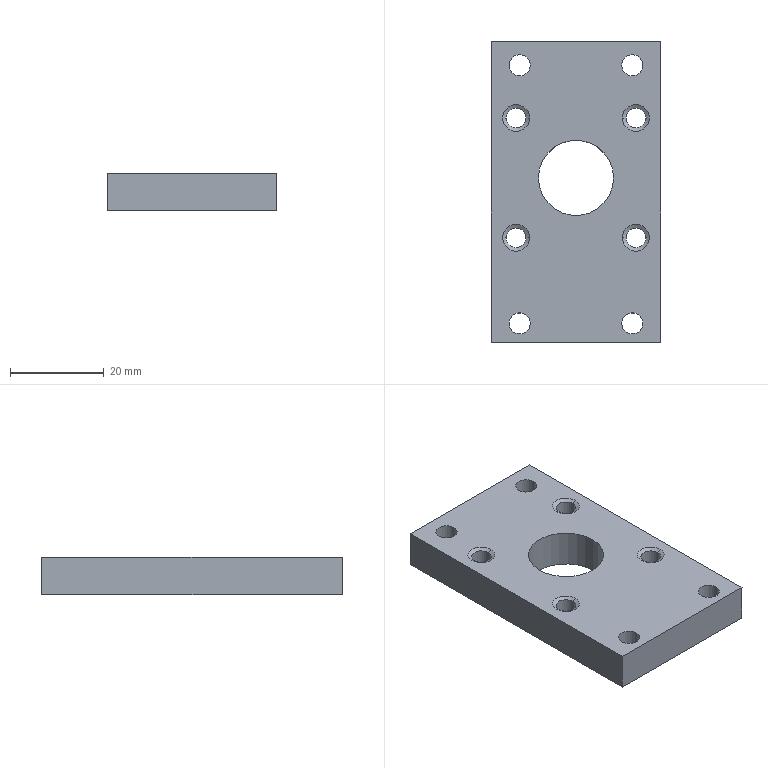Part | NX | 1 solid | 32 faces | box 36.002 x 64 x 8.011 mm | volume 15861 mm3 | cylinder 18 | cone 8 | plane 6 | commonest cylinder face diameters 4.2 x8 4.5 x8 16 x2
STEP:
#1=CARTESIAN_POINT('',(1234.583,117.5,67.602));
#2=VERTEX_POINT('',#1);
#3=CARTESIAN_POINT('',(1198.583,117.5,67.613));
#4=VERTEX_POINT('',#3);
#5=CARTESIAN_POINT('',(1211.755,117.5,67.609));
#6=DIRECTION('',(-1.,0.,0.0003046));
#7=VECTOR('',#6,1000.);
#8=LINE('',#5,#7);
#9=EDGE_CURVE('',#2,#4,#8,.T.);
#10=ORIENTED_EDGE('',*,*,#9,.F.);
#11=CARTESIAN_POINT('',(1234.585,117.5,75.602));
#12=VERTEX_POINT('',#11);
#13=CARTESIAN_POINT('',(1234.582,117.5,65.602));
#14=DIRECTION('',(0.0003046,0.,1.));
#15=VECTOR('',#14,1000.);
#16=LINE('',#13,#15);
#17=EDGE_CURVE('',#2,#12,#16,.T.);
#18=ORIENTED_EDGE('',*,*,#17,.T.);
#19=CARTESIAN_POINT('',(1198.585,117.5,75.613));
#20=VERTEX_POINT('',#19);
#21=CARTESIAN_POINT('',(1211.758,117.5,75.609));
#22=DIRECTION('',(-1.,0.,0.0003046));
#23=VECTOR('',#22,1000.);
#24=LINE('',#21,#23);
#25=EDGE_CURVE('',#12,#20,#24,.T.);
#26=ORIENTED_EDGE('',*,*,#25,.T.);
#27=CARTESIAN_POINT('',(1198.582,117.5,65.613));
#28=DIRECTION('',(-0.0003046,0.,-1.));
#29=VECTOR('',#28,1000.);
#30=LINE('',#27,#29);
#31=EDGE_CURVE('',#20,#4,#30,.T.);
#32=ORIENTED_EDGE('',*,*,#31,.T.);
#33=EDGE_LOOP('',(#10,#18,#26,#32));
#34=FACE_BOUND('',#33,.T.);
#35=CARTESIAN_POINT('',(1236.582,117.5,65.601));
#36=DIRECTION('',(0.,-1.,0.));
#37=DIRECTION('',(0.,0.,-1.));
#38=AXIS2_PLACEMENT_3D('',#35,#36,#37);
#39=PLANE('',#38);
#40=ADVANCED_FACE('',(#34),#39,.T.);
#41=CARTESIAN_POINT('',(1234.583,181.5,67.602));
#42=VERTEX_POINT('',#41);
#43=CARTESIAN_POINT('',(1234.583,131.898,67.602));
#44=DIRECTION('',(0.,-1.,0.));
#45=VECTOR('',#44,1000.);
#46=LINE('',#43,#45);
#47=EDGE_CURVE('',#42,#2,#46,.T.);
#48=ORIENTED_EDGE('',*,*,#47,.F.);
#49=CARTESIAN_POINT('',(1234.585,181.5,75.602));
#50=VERTEX_POINT('',#49);
#51=CARTESIAN_POINT('',(1234.582,181.5,65.602));
#52=DIRECTION('',(0.0003046,0.,1.));
#53=VECTOR('',#52,1000.);
#54=LINE('',#51,#53);
#55=EDGE_CURVE('',#42,#50,#54,.T.);
#56=ORIENTED_EDGE('',*,*,#55,.T.);
#57=CARTESIAN_POINT('',(1234.585,131.898,75.602));
#58=DIRECTION('',(0.,-1.,0.));
#59=VECTOR('',#58,1000.);
#60=LINE('',#57,#59);
#61=EDGE_CURVE('',#50,#12,#60,.T.);
#62=ORIENTED_EDGE('',*,*,#61,.T.);
#63=ORIENTED_EDGE('',*,*,#17,.F.);
#64=EDGE_LOOP('',(#48,#56,#62,#63));
#65=FACE_BOUND('',#64,.T.);
#66=CARTESIAN_POINT('',(1234.582,127.5,65.602));
#67=DIRECTION('',(1.,0.,-0.0003046));
#68=DIRECTION('',(0.,-1.,0.));
#69=AXIS2_PLACEMENT_3D('',#66,#67,#68);
#70=PLANE('',#69);
#71=ADVANCED_FACE('',(#65),#70,.T.);
#72=CARTESIAN_POINT('',(1198.583,181.5,67.613));
#73=VERTEX_POINT('',#72);
#74=CARTESIAN_POINT('',(1211.755,181.5,67.609));
#75=DIRECTION('',(1.,0.,-0.0003046));
#76=VECTOR('',#75,1000.);
#77=LINE('',#74,#76);
#78=EDGE_CURVE('',#73,#42,#77,.T.);
#79=ORIENTED_EDGE('',*,*,#78,.F.);
#80=CARTESIAN_POINT('',(1198.585,181.5,75.613));
#81=VERTEX_POINT('',#80);
#82=CARTESIAN_POINT('',(1198.582,181.5,65.613));
#83=DIRECTION('',(-0.0003046,0.,-1.));
#84=VECTOR('',#83,1000.);
#85=LINE('',#82,#84);
#86=EDGE_CURVE('',#81,#73,#85,.T.);
#87=ORIENTED_EDGE('',*,*,#86,.F.);
#88=CARTESIAN_POINT('',(1211.758,181.5,75.609));
#89=DIRECTION('',(1.,0.,-0.0003046));
#90=VECTOR('',#89,1000.);
#91=LINE('',#88,#90);
#92=EDGE_CURVE('',#81,#50,#91,.T.);
#93=ORIENTED_EDGE('',*,*,#92,.T.);
#94=ORIENTED_EDGE('',*,*,#55,.F.);
#95=EDGE_LOOP('',(#79,#87,#93,#94));
#96=FACE_BOUND('',#95,.T.);
#97=CARTESIAN_POINT('',(1196.582,181.5,65.614));
#98=DIRECTION('',(0.,1.,0.));
#99=DIRECTION('',(0.,0.,-1.));
#100=AXIS2_PLACEMENT_3D('',#97,#98,#99);
#101=PLANE('',#100);
#102=ADVANCED_FACE('',(#96),#101,.T.);
#103=CARTESIAN_POINT('',(1198.583,131.898,67.613));
#104=DIRECTION('',(0.,1.,0.));
#105=VECTOR('',#104,1000.);
#106=LINE('',#103,#105);
#107=EDGE_CURVE('',#4,#73,#106,.T.);
#108=ORIENTED_EDGE('',*,*,#107,.F.);
#109=ORIENTED_EDGE('',*,*,#31,.F.);
#110=CARTESIAN_POINT('',(1198.585,131.898,75.613));
#111=DIRECTION('',(0.,1.,0.));
#112=VECTOR('',#111,1000.);
#113=LINE('',#110,#112);
#114=EDGE_CURVE('',#20,#81,#113,.T.);
#115=ORIENTED_EDGE('',*,*,#114,.T.);
#116=ORIENTED_EDGE('',*,*,#86,.T.);
#117=EDGE_LOOP('',(#108,#109,#115,#116));
#118=FACE_BOUND('',#117,.T.);
#119=CARTESIAN_POINT('',(1198.582,117.5,65.613));
#120=DIRECTION('',(-1.,0.,0.0003046));
#121=DIRECTION('',(0.,1.,0.));
#122=AXIS2_PLACEMENT_3D('',#119,#120,#121);
#123=PLANE('',#122);
#124=ADVANCED_FACE('',(#118),#123,.T.);
#125=ORIENTED_EDGE('',*,*,#61,.F.);
#126=ORIENTED_EDGE('',*,*,#92,.F.);
#127=ORIENTED_EDGE('',*,*,#114,.F.);
#128=ORIENTED_EDGE('',*,*,#25,.F.);
#129=EDGE_LOOP('',(#125,#126,#127,#128));
#130=FACE_BOUND('',#129,.T.);
#131=CARTESIAN_POINT('',(1224.585,152.5,75.605));
#132=VERTEX_POINT('',#131);
#133=CARTESIAN_POINT('',(1208.585,152.5,75.61));
#134=VERTEX_POINT('',#133);
#135=CARTESIAN_POINT('',(1216.585,152.5,75.608));
#136=DIRECTION('',(-0.0003046,0.,-1.));
#137=DIRECTION('',(-1.,0.,0.0003046));
#138=AXIS2_PLACEMENT_3D('',#135,#136,#137);
#139=CIRCLE('',#138,8.);
#140=EDGE_CURVE('',#132,#134,#139,.T.);
#141=ORIENTED_EDGE('',*,*,#140,.T.);
#142=CARTESIAN_POINT('',(1216.585,152.5,75.608));
#143=DIRECTION('',(-0.0003046,0.,-1.));
#144=DIRECTION('',(-1.,0.,0.0003046));
#145=AXIS2_PLACEMENT_3D('',#142,#143,#144);
#146=CIRCLE('',#145,8.);
#147=EDGE_CURVE('',#134,#132,#146,.T.);
#148=ORIENTED_EDGE('',*,*,#147,.T.);
#149=EDGE_LOOP('',(#141,#148));
#150=FACE_BOUND('',#149,.T.);
#151=CARTESIAN_POINT('',(1226.475,165.25,75.605));
#152=VERTEX_POINT('',#151);
#153=CARTESIAN_POINT('',(1232.195,165.25,75.603));
#154=VERTEX_POINT('',#153);
#155=CARTESIAN_POINT('',(1229.335,165.25,75.604));
#156=DIRECTION('',(0.0003046,0.,1.));
#157=DIRECTION('',(1.,0.,-0.0003046));
#158=AXIS2_PLACEMENT_3D('',#155,#156,#157);
#159=CIRCLE('',#158,2.86);
#160=EDGE_CURVE('',#152,#154,#159,.T.);
#161=ORIENTED_EDGE('',*,*,#160,.F.);
#162=CARTESIAN_POINT('',(1229.335,165.25,75.604));
#163=DIRECTION('',(0.0003046,0.,1.));
#164=DIRECTION('',(1.,0.,-0.0003046));
#165=AXIS2_PLACEMENT_3D('',#162,#163,#164);
#166=CIRCLE('',#165,2.86);
#167=EDGE_CURVE('',#154,#152,#166,.T.);
#168=ORIENTED_EDGE('',*,*,#167,.F.);
#169=EDGE_LOOP('',(#161,#168));
#170=FACE_BOUND('',#169,.T.);
#171=CARTESIAN_POINT('',(1232.195,139.75,75.603));
#172=VERTEX_POINT('',#171);
#173=CARTESIAN_POINT('',(1226.475,139.75,75.605));
#174=VERTEX_POINT('',#173);
#175=CARTESIAN_POINT('',(1229.335,139.75,75.604));
#176=DIRECTION('',(0.0003046,0.,1.));
#177=DIRECTION('',(1.,0.,-0.0003046));
#178=AXIS2_PLACEMENT_3D('',#175,#176,#177);
#179=CIRCLE('',#178,2.86);
#180=EDGE_CURVE('',#172,#174,#179,.T.);
#181=ORIENTED_EDGE('',*,*,#180,.F.);
#182=CARTESIAN_POINT('',(1229.335,139.75,75.604));
#183=DIRECTION('',(0.0003046,0.,1.));
#184=DIRECTION('',(1.,0.,-0.0003046));
#185=AXIS2_PLACEMENT_3D('',#182,#183,#184);
#186=CIRCLE('',#185,2.86);
#187=EDGE_CURVE('',#174,#172,#186,.T.);
#188=ORIENTED_EDGE('',*,*,#187,.F.);
#189=EDGE_LOOP('',(#181,#188));
#190=FACE_BOUND('',#189,.T.);
#191=CARTESIAN_POINT('',(1226.335,121.5,75.605));
#192=VERTEX_POINT('',#191);
#193=CARTESIAN_POINT('',(1230.835,121.5,75.603));
#194=VERTEX_POINT('',#193);
#195=CARTESIAN_POINT('',(1228.585,121.5,75.604));
#196=DIRECTION('',(0.0003046,0.,1.));
#197=DIRECTION('',(1.,0.,-0.0003046));
#198=AXIS2_PLACEMENT_3D('',#195,#196,#197);
#199=CIRCLE('',#198,2.25);
#200=EDGE_CURVE('',#192,#194,#199,.T.);
#201=ORIENTED_EDGE('',*,*,#200,.F.);
#202=CARTESIAN_POINT('',(1228.585,121.5,75.604));
#203=DIRECTION('',(0.0003046,0.,1.));
#204=DIRECTION('',(1.,0.,-0.0003046));
#205=AXIS2_PLACEMENT_3D('',#202,#203,#204);
#206=CIRCLE('',#205,2.25);
#207=EDGE_CURVE('',#194,#192,#206,.T.);
#208=ORIENTED_EDGE('',*,*,#207,.F.);
#209=EDGE_LOOP('',(#201,#208));
#210=FACE_BOUND('',#209,.T.);
#211=CARTESIAN_POINT('',(1202.335,121.5,75.612));
#212=VERTEX_POINT('',#211);
#213=CARTESIAN_POINT('',(1206.835,121.5,75.611));
#214=VERTEX_POINT('',#213);
#215=CARTESIAN_POINT('',(1204.585,121.5,75.611));
#216=DIRECTION('',(0.0003046,0.,1.));
#217=DIRECTION('',(1.,0.,-0.0003046));
#218=AXIS2_PLACEMENT_3D('',#215,#216,#217);
#219=CIRCLE('',#218,2.25);
#220=EDGE_CURVE('',#212,#214,#219,.T.);
#221=ORIENTED_EDGE('',*,*,#220,.F.);
#222=CARTESIAN_POINT('',(1204.585,121.5,75.611));
#223=DIRECTION('',(0.0003046,0.,1.));
#224=DIRECTION('',(1.,0.,-0.0003046));
#225=AXIS2_PLACEMENT_3D('',#222,#223,#224);
#226=CIRCLE('',#225,2.25);
#227=EDGE_CURVE('',#214,#212,#226,.T.);
#228=ORIENTED_EDGE('',*,*,#227,.F.);
#229=EDGE_LOOP('',(#221,#228));
#230=FACE_BOUND('',#229,.T.);
#231=CARTESIAN_POINT('',(1202.335,176.5,75.612));
#232=VERTEX_POINT('',#231);
#233=CARTESIAN_POINT('',(1206.835,176.5,75.611));
#234=VERTEX_POINT('',#233);
#235=CARTESIAN_POINT('',(1204.585,176.5,75.611));
#236=DIRECTION('',(0.0003046,0.,1.));
#237=DIRECTION('',(1.,0.,-0.0003046));
#238=AXIS2_PLACEMENT_3D('',#235,#236,#237);
#239=CIRCLE('',#238,2.25);
#240=EDGE_CURVE('',#232,#234,#239,.T.);
#241=ORIENTED_EDGE('',*,*,#240,.F.);
#242=CARTESIAN_POINT('',(1204.585,176.5,75.611));
#243=DIRECTION('',(0.0003046,0.,1.));
#244=DIRECTION('',(1.,0.,-0.0003046));
#245=AXIS2_PLACEMENT_3D('',#242,#243,#244);
#246=CIRCLE('',#245,2.25);
#247=EDGE_CURVE('',#234,#232,#246,.T.);
#248=ORIENTED_EDGE('',*,*,#247,.F.);
#249=EDGE_LOOP('',(#241,#248));
#250=FACE_BOUND('',#249,.T.);
#251=CARTESIAN_POINT('',(1230.835,176.5,75.603));
#252=VERTEX_POINT('',#251);
#253=CARTESIAN_POINT('',(1226.335,176.5,75.605));
#254=VERTEX_POINT('',#253);
#255=CARTESIAN_POINT('',(1228.585,176.5,75.604));
#256=DIRECTION('',(0.0003046,0.,1.));
#257=DIRECTION('',(1.,0.,-0.0003046));
#258=AXIS2_PLACEMENT_3D('',#255,#256,#257);
#259=CIRCLE('',#258,2.25);
#260=EDGE_CURVE('',#252,#254,#259,.T.);
#261=ORIENTED_EDGE('',*,*,#260,.F.);
#262=CARTESIAN_POINT('',(1228.585,176.5,75.604));
#263=DIRECTION('',(0.0003046,0.,1.));
#264=DIRECTION('',(1.,0.,-0.0003046));
#265=AXIS2_PLACEMENT_3D('',#262,#263,#264);
#266=CIRCLE('',#265,2.25);
#267=EDGE_CURVE('',#254,#252,#266,.T.);
#268=ORIENTED_EDGE('',*,*,#267,.F.);
#269=EDGE_LOOP('',(#261,#268));
#270=FACE_BOUND('',#269,.T.);
#271=CARTESIAN_POINT('',(1206.695,139.75,75.611));
#272=VERTEX_POINT('',#271);
#273=CARTESIAN_POINT('',(1200.975,139.75,75.612));
#274=VERTEX_POINT('',#273);
#275=CARTESIAN_POINT('',(1203.835,139.75,75.611));
#276=DIRECTION('',(0.0003046,0.,1.));
#277=DIRECTION('',(1.,0.,-0.0003046));
#278=AXIS2_PLACEMENT_3D('',#275,#276,#277);
#279=CIRCLE('',#278,2.86);
#280=EDGE_CURVE('',#272,#274,#279,.T.);
#281=ORIENTED_EDGE('',*,*,#280,.F.);
#282=CARTESIAN_POINT('',(1203.835,139.75,75.611));
#283=DIRECTION('',(0.0003046,0.,1.));
#284=DIRECTION('',(1.,0.,-0.0003046));
#285=AXIS2_PLACEMENT_3D('',#282,#283,#284);
#286=CIRCLE('',#285,2.86);
#287=EDGE_CURVE('',#274,#272,#286,.T.);
#288=ORIENTED_EDGE('',*,*,#287,.F.);
#289=EDGE_LOOP('',(#281,#288));
#290=FACE_BOUND('',#289,.T.);
#291=CARTESIAN_POINT('',(1200.975,165.25,75.612));
#292=VERTEX_POINT('',#291);
#293=CARTESIAN_POINT('',(1206.695,165.25,75.611));
#294=VERTEX_POINT('',#293);
#295=CARTESIAN_POINT('',(1203.835,165.25,75.611));
#296=DIRECTION('',(0.0003046,0.,1.));
#297=DIRECTION('',(1.,0.,-0.0003046));
#298=AXIS2_PLACEMENT_3D('',#295,#296,#297);
#299=CIRCLE('',#298,2.86);
#300=EDGE_CURVE('',#292,#294,#299,.T.);
#301=ORIENTED_EDGE('',*,*,#300,.F.);
#302=CARTESIAN_POINT('',(1203.835,165.25,75.611));
#303=DIRECTION('',(0.0003046,0.,1.));
#304=DIRECTION('',(1.,0.,-0.0003046));
#305=AXIS2_PLACEMENT_3D('',#302,#303,#304);
#306=CIRCLE('',#305,2.86);
#307=EDGE_CURVE('',#294,#292,#306,.T.);
#308=ORIENTED_EDGE('',*,*,#307,.F.);
#309=EDGE_LOOP('',(#301,#308));
#310=FACE_BOUND('',#309,.T.);
#311=CARTESIAN_POINT('',(1211.758,131.898,75.609));
#312=DIRECTION('',(0.0003046,0.,1.));
#313=DIRECTION('',(-0.000000134,-1.,0.));
#314=AXIS2_PLACEMENT_3D('',#311,#312,#313);
#315=PLANE('',#314);
#316=ADVANCED_FACE('',(#130,#150,#170,#190,#210,#230,#250,#270,#290,#310),#315,.T.);
#317=ORIENTED_EDGE('',*,*,#140,.F.);
#318=CARTESIAN_POINT('',(1224.583,152.5,67.605));
#319=VERTEX_POINT('',#318);
#320=CARTESIAN_POINT('',(1224.585,152.5,76.62));
#321=DIRECTION('',(-0.0003046,0.,-1.));
#322=VECTOR('',#321,1000.);
#323=LINE('',#320,#322);
#324=EDGE_CURVE('',#319,#132,#323,.F.);
#325=ORIENTED_EDGE('',*,*,#324,.F.);
#326=CARTESIAN_POINT('',(1208.583,152.5,67.61));
#327=VERTEX_POINT('',#326);
#328=CARTESIAN_POINT('',(1216.583,152.5,67.608));
#329=DIRECTION('',(-0.0003046,0.,-1.));
#330=DIRECTION('',(-1.,0.,0.0003046));
#331=AXIS2_PLACEMENT_3D('',#328,#329,#330);
#332=CIRCLE('',#331,8.);
#333=EDGE_CURVE('',#319,#327,#332,.T.);
#334=ORIENTED_EDGE('',*,*,#333,.T.);
#335=CARTESIAN_POINT('',(1208.585,152.5,76.625));
#336=DIRECTION('',(-0.0003046,0.,-1.));
#337=VECTOR('',#336,1000.);
#338=LINE('',#335,#337);
#339=EDGE_CURVE('',#327,#134,#338,.F.);
#340=ORIENTED_EDGE('',*,*,#339,.T.);
#341=EDGE_LOOP('',(#317,#325,#334,#340));
#342=FACE_BOUND('',#341,.T.);
#343=CARTESIAN_POINT('',(1216.585,152.5,76.622));
#344=DIRECTION('',(-0.0003046,0.,-1.));
#345=DIRECTION('',(-1.,0.,0.0003046));
#346=AXIS2_PLACEMENT_3D('',#343,#344,#345);
#347=CYLINDRICAL_SURFACE('',#346,8.);
#348=ADVANCED_FACE('',(#342),#347,.F.);
#349=ORIENTED_EDGE('',*,*,#240,.T.);
#350=CARTESIAN_POINT('',(1206.833,176.5,67.611));
#351=VERTEX_POINT('',#350);
#352=CARTESIAN_POINT('',(1206.832,176.5,66.797));
#353=DIRECTION('',(0.0003046,0.,1.));
#354=VECTOR('',#353,1000.);
#355=LINE('',#352,#354);
#356=EDGE_CURVE('',#351,#234,#355,.T.);
#357=ORIENTED_EDGE('',*,*,#356,.F.);
#358=CARTESIAN_POINT('',(1202.333,176.5,67.612));
#359=VERTEX_POINT('',#358);
#360=CARTESIAN_POINT('',(1204.583,176.5,67.611));
#361=DIRECTION('',(0.0003046,0.,1.));
#362=DIRECTION('',(1.,0.,-0.0003046));
#363=AXIS2_PLACEMENT_3D('',#360,#361,#362);
#364=CIRCLE('',#363,2.25);
#365=EDGE_CURVE('',#359,#351,#364,.T.);
#366=ORIENTED_EDGE('',*,*,#365,.F.);
#367=CARTESIAN_POINT('',(1202.332,176.5,66.799));
#368=DIRECTION('',(0.0003046,0.,1.));
#369=VECTOR('',#368,1000.);
#370=LINE('',#367,#369);
#371=EDGE_CURVE('',#359,#232,#370,.T.);
#372=ORIENTED_EDGE('',*,*,#371,.T.);
#373=EDGE_LOOP('',(#349,#357,#366,#372));
#374=FACE_BOUND('',#373,.T.);
#375=CARTESIAN_POINT('',(1204.582,176.5,66.798));
#376=DIRECTION('',(0.0003046,0.,1.));
#377=DIRECTION('',(1.,0.,-0.0003046));
#378=AXIS2_PLACEMENT_3D('',#375,#376,#377);
#379=CYLINDRICAL_SURFACE('',#378,2.25);
#380=ADVANCED_FACE('',(#374),#379,.F.);
#381=CARTESIAN_POINT('',(1230.833,176.5,67.603));
#382=VERTEX_POINT('',#381);
#383=CARTESIAN_POINT('',(1226.333,176.5,67.605));
#384=VERTEX_POINT('',#383);
#385=CARTESIAN_POINT('',(1228.583,176.5,67.604));
#386=DIRECTION('',(0.0003046,0.,1.));
#387=DIRECTION('',(1.,0.,-0.0003046));
#388=AXIS2_PLACEMENT_3D('',#385,#386,#387);
#389=CIRCLE('',#388,2.25);
#390=EDGE_CURVE('',#382,#384,#389,.T.);
#391=ORIENTED_EDGE('',*,*,#390,.F.);
#392=CARTESIAN_POINT('',(1230.832,176.5,66.79));
#393=DIRECTION('',(0.0003046,0.,1.));
#394=VECTOR('',#393,1000.);
#395=LINE('',#392,#394);
#396=EDGE_CURVE('',#382,#252,#395,.T.);
#397=ORIENTED_EDGE('',*,*,#396,.T.);
#398=ORIENTED_EDGE('',*,*,#260,.T.);
#399=CARTESIAN_POINT('',(1226.332,176.5,66.791));
#400=DIRECTION('',(0.0003046,0.,1.));
#401=VECTOR('',#400,1000.);
#402=LINE('',#399,#401);
#403=EDGE_CURVE('',#384,#254,#402,.T.);
#404=ORIENTED_EDGE('',*,*,#403,.F.);
#405=EDGE_LOOP('',(#391,#397,#398,#404));
#406=FACE_BOUND('',#405,.T.);
#407=CARTESIAN_POINT('',(1228.582,176.5,66.791));
#408=DIRECTION('',(0.0003046,0.,1.));
#409=DIRECTION('',(1.,0.,-0.0003046));
#410=AXIS2_PLACEMENT_3D('',#407,#408,#409);
#411=CYLINDRICAL_SURFACE('',#410,2.25);
#412=ADVANCED_FACE('',(#406),#411,.F.);
#413=CARTESIAN_POINT('',(1206.833,121.5,67.611));
#414=VERTEX_POINT('',#413);
#415=CARTESIAN_POINT('',(1202.333,121.5,67.612));
#416=VERTEX_POINT('',#415);
#417=CARTESIAN_POINT('',(1204.583,121.5,67.611));
#418=DIRECTION('',(0.0003046,0.,1.));
#419=DIRECTION('',(1.,0.,-0.0003046));
#420=AXIS2_PLACEMENT_3D('',#417,#418,#419);
#421=CIRCLE('',#420,2.25);
#422=EDGE_CURVE('',#414,#416,#421,.T.);
#423=ORIENTED_EDGE('',*,*,#422,.F.);
#424=CARTESIAN_POINT('',(1206.832,121.5,64.596));
#425=DIRECTION('',(0.0003046,0.,1.));
#426=VECTOR('',#425,1000.);
#427=LINE('',#424,#426);
#428=EDGE_CURVE('',#414,#214,#427,.T.);
#429=ORIENTED_EDGE('',*,*,#428,.T.);
#430=ORIENTED_EDGE('',*,*,#227,.T.);
#431=CARTESIAN_POINT('',(1202.332,121.5,64.597));
#432=DIRECTION('',(0.0003046,0.,1.));
#433=VECTOR('',#432,1000.);
#434=LINE('',#431,#433);
#435=EDGE_CURVE('',#416,#212,#434,.T.);
#436=ORIENTED_EDGE('',*,*,#435,.F.);
#437=EDGE_LOOP('',(#423,#429,#430,#436));
#438=FACE_BOUND('',#437,.T.);
#439=CARTESIAN_POINT('',(1204.582,121.5,64.597));
#440=DIRECTION('',(0.0003046,0.,1.));
#441=DIRECTION('',(1.,0.,-0.0003046));
#442=AXIS2_PLACEMENT_3D('',#439,#440,#441);
#443=CYLINDRICAL_SURFACE('',#442,2.25);
#444=ADVANCED_FACE('',(#438),#443,.F.);
#445=ORIENTED_EDGE('',*,*,#200,.T.);
#446=CARTESIAN_POINT('',(1230.833,121.5,67.603));
#447=VERTEX_POINT('',#446);
#448=CARTESIAN_POINT('',(1230.832,121.5,64.589));
#449=DIRECTION('',(0.0003046,0.,1.));
#450=VECTOR('',#449,1000.);
#451=LINE('',#448,#450);
#452=EDGE_CURVE('',#447,#194,#451,.T.);
#453=ORIENTED_EDGE('',*,*,#452,.F.);
#454=CARTESIAN_POINT('',(1226.333,121.5,67.605));
#455=VERTEX_POINT('',#454);
#456=CARTESIAN_POINT('',(1228.583,121.5,67.604));
#457=DIRECTION('',(0.0003046,0.,1.));
#458=DIRECTION('',(1.,0.,-0.0003046));
#459=AXIS2_PLACEMENT_3D('',#456,#457,#458);
#460=CIRCLE('',#459,2.25);
#461=EDGE_CURVE('',#455,#447,#460,.T.);
#462=ORIENTED_EDGE('',*,*,#461,.F.);
#463=CARTESIAN_POINT('',(1226.332,121.5,64.59));
#464=DIRECTION('',(0.0003046,0.,1.));
#465=VECTOR('',#464,1000.);
#466=LINE('',#463,#465);
#467=EDGE_CURVE('',#455,#192,#466,.T.);
#468=ORIENTED_EDGE('',*,*,#467,.T.);
#469=EDGE_LOOP('',(#445,#453,#462,#468));
#470=FACE_BOUND('',#469,.T.);
#471=CARTESIAN_POINT('',(1228.582,121.5,64.589));
#472=DIRECTION('',(0.0003046,0.,1.));
#473=DIRECTION('',(1.,0.,-0.0003046));
#474=AXIS2_PLACEMENT_3D('',#471,#472,#473);
#475=CYLINDRICAL_SURFACE('',#474,2.25);
#476=ADVANCED_FACE('',(#470),#475,.F.);
#477=CARTESIAN_POINT('',(1205.935,139.75,75.172));
#478=VERTEX_POINT('',#477);
#479=CARTESIAN_POINT('',(1201.735,139.75,75.173));
#480=VERTEX_POINT('',#479);
#481=CARTESIAN_POINT('',(1203.835,139.75,75.173));
#482=DIRECTION('',(0.0003046,0.,1.));
#483=DIRECTION('',(1.,0.,-0.0003046));
#484=AXIS2_PLACEMENT_3D('',#481,#482,#483);
#485=CIRCLE('',#484,2.1);
#486=EDGE_CURVE('',#478,#480,#485,.T.);
#487=ORIENTED_EDGE('',*,*,#486,.T.);
#488=CARTESIAN_POINT('',(1201.733,139.75,67.612));
#489=VERTEX_POINT('',#488);
#490=CARTESIAN_POINT('',(1201.735,139.75,75.612));
#491=DIRECTION('',(0.0003046,0.,1.));
#492=VECTOR('',#491,1000.);
#493=LINE('',#490,#492);
#494=EDGE_CURVE('',#480,#489,#493,.F.);
#495=ORIENTED_EDGE('',*,*,#494,.T.);
#496=CARTESIAN_POINT('',(1205.933,139.75,67.611));
#497=VERTEX_POINT('',#496);
#498=CARTESIAN_POINT('',(1203.833,139.75,67.611));
#499=DIRECTION('',(0.0003046,0.,1.));
#500=DIRECTION('',(1.,0.,-0.0003046));
#501=AXIS2_PLACEMENT_3D('',#498,#499,#500);
#502=CIRCLE('',#501,2.1);
#503=EDGE_CURVE('',#497,#489,#502,.T.);
#504=ORIENTED_EDGE('',*,*,#503,.F.);
#505=CARTESIAN_POINT('',(1205.935,139.75,75.611));
#506=DIRECTION('',(0.0003046,0.,1.));
#507=VECTOR('',#506,1000.);
#508=LINE('',#505,#507);
#509=EDGE_CURVE('',#478,#497,#508,.F.);
#510=ORIENTED_EDGE('',*,*,#509,.F.);
#511=EDGE_LOOP('',(#487,#495,#504,#510));
#512=FACE_BOUND('',#511,.T.);
#513=CARTESIAN_POINT('',(1203.835,139.75,75.611));
#514=DIRECTION('',(0.0003046,0.,1.));
#515=DIRECTION('',(1.,0.,-0.0003046));
#516=AXIS2_PLACEMENT_3D('',#513,#514,#515);
#517=CYLINDRICAL_SURFACE('',#516,2.1);
#518=ADVANCED_FACE('',(#512),#517,.F.);
#519=ORIENTED_EDGE('',*,*,#280,.T.);
#520=CARTESIAN_POINT('',(1201.735,139.75,75.173));
#521=DIRECTION('',(-0.8659,0.,0.5003));
#522=VECTOR('',#521,1000.);
#523=LINE('',#520,#522);
#524=EDGE_CURVE('',#480,#274,#523,.T.);
#525=ORIENTED_EDGE('',*,*,#524,.F.);
#526=ORIENTED_EDGE('',*,*,#486,.F.);
#527=CARTESIAN_POINT('',(1205.935,139.75,75.172));
#528=DIRECTION('',(0.8662,0.,0.4997));
#529=VECTOR('',#528,1000.);
#530=LINE('',#527,#529);
#531=EDGE_CURVE('',#478,#272,#530,.T.);
#532=ORIENTED_EDGE('',*,*,#531,.T.);
#533=EDGE_LOOP('',(#519,#525,#526,#532));
#534=FACE_BOUND('',#533,.T.);
#535=CARTESIAN_POINT('',(1203.835,139.75,75.173));
#536=DIRECTION('',(0.0003046,0.,1.));
#537=DIRECTION('',(1.,0.,-0.0003046));
#538=AXIS2_PLACEMENT_3D('',#535,#536,#537);
#539=CONICAL_SURFACE('',#538,2.1,1.047);
#540=ADVANCED_FACE('',(#534),#539,.F.);
#541=CARTESIAN_POINT('',(1231.433,139.75,67.603));
#542=VERTEX_POINT('',#541);
#543=CARTESIAN_POINT('',(1227.233,139.75,67.604));
#544=VERTEX_POINT('',#543);
#545=CARTESIAN_POINT('',(1229.333,139.75,67.604));
#546=DIRECTION('',(0.0003046,0.,1.));
#547=DIRECTION('',(1.,0.,-0.0003046));
#548=AXIS2_PLACEMENT_3D('',#545,#546,#547);
#549=CIRCLE('',#548,2.1);
#550=EDGE_CURVE('',#542,#544,#549,.T.);
#551=ORIENTED_EDGE('',*,*,#550,.F.);
#552=CARTESIAN_POINT('',(1231.435,139.75,75.164));
#553=VERTEX_POINT('',#552);
#554=CARTESIAN_POINT('',(1231.435,139.75,75.603));
#555=DIRECTION('',(0.0003046,0.,1.));
#556=VECTOR('',#555,1000.);
#557=LINE('',#554,#556);
#558=EDGE_CURVE('',#542,#553,#557,.T.);
#559=ORIENTED_EDGE('',*,*,#558,.T.);
#560=CARTESIAN_POINT('',(1227.235,139.75,75.166));
#561=VERTEX_POINT('',#560);
#562=CARTESIAN_POINT('',(1229.335,139.75,75.165));
#563=DIRECTION('',(0.0003046,0.,1.));
#564=DIRECTION('',(1.,0.,-0.0003046));
#565=AXIS2_PLACEMENT_3D('',#562,#563,#564);
#566=CIRCLE('',#565,2.1);
#567=EDGE_CURVE('',#553,#561,#566,.T.);
#568=ORIENTED_EDGE('',*,*,#567,.T.);
#569=CARTESIAN_POINT('',(1227.235,139.75,75.604));
#570=DIRECTION('',(0.0003046,0.,1.));
#571=VECTOR('',#570,1000.);
#572=LINE('',#569,#571);
#573=EDGE_CURVE('',#544,#561,#572,.T.);
#574=ORIENTED_EDGE('',*,*,#573,.F.);
#575=EDGE_LOOP('',(#551,#559,#568,#574));
#576=FACE_BOUND('',#575,.T.);
#577=CARTESIAN_POINT('',(1229.335,139.75,75.604));
#578=DIRECTION('',(0.0003046,0.,1.));
#579=DIRECTION('',(1.,0.,-0.0003046));
#580=AXIS2_PLACEMENT_3D('',#577,#578,#579);
#581=CYLINDRICAL_SURFACE('',#580,2.1);
#582=ADVANCED_FACE('',(#576),#581,.F.);
#583=CARTESIAN_POINT('',(1229.335,139.75,75.165));
#584=DIRECTION('',(0.0003046,0.,1.));
#585=DIRECTION('',(1.,0.,-0.0003046));
#586=AXIS2_PLACEMENT_3D('',#583,#584,#585);
#587=CIRCLE('',#586,2.1);
#588=EDGE_CURVE('',#561,#553,#587,.T.);
#589=ORIENTED_EDGE('',*,*,#588,.F.);
#590=CARTESIAN_POINT('',(1227.235,139.75,75.166));
#591=DIRECTION('',(-0.8659,0.,0.5003));
#592=VECTOR('',#591,1000.);
#593=LINE('',#590,#592);
#594=EDGE_CURVE('',#174,#561,#593,.F.);
#595=ORIENTED_EDGE('',*,*,#594,.F.);
#596=ORIENTED_EDGE('',*,*,#187,.T.);
#597=CARTESIAN_POINT('',(1231.435,139.75,75.164));
#598=DIRECTION('',(0.8662,0.,0.4997));
#599=VECTOR('',#598,1000.);
#600=LINE('',#597,#599);
#601=EDGE_CURVE('',#172,#553,#600,.F.);
#602=ORIENTED_EDGE('',*,*,#601,.T.);
#603=EDGE_LOOP('',(#589,#595,#596,#602));
#604=FACE_BOUND('',#603,.T.);
#605=CARTESIAN_POINT('',(1229.335,139.75,75.165));
#606=DIRECTION('',(0.0003046,0.,1.));
#607=DIRECTION('',(1.,0.,-0.0003046));
#608=AXIS2_PLACEMENT_3D('',#605,#606,#607);
#609=CONICAL_SURFACE('',#608,2.1,1.047);
#610=ADVANCED_FACE('',(#604),#609,.F.);
#611=CARTESIAN_POINT('',(1205.935,165.25,75.172));
#612=VERTEX_POINT('',#611);
#613=CARTESIAN_POINT('',(1201.735,165.25,75.173));
#614=VERTEX_POINT('',#613);
#615=CARTESIAN_POINT('',(1203.835,165.25,75.173));
#616=DIRECTION('',(0.0003046,0.,1.));
#617=DIRECTION('',(1.,0.,-0.0003046));
#618=AXIS2_PLACEMENT_3D('',#615,#616,#617);
#619=CIRCLE('',#618,2.1);
#620=EDGE_CURVE('',#612,#614,#619,.T.);
#621=ORIENTED_EDGE('',*,*,#620,.T.);
#622=CARTESIAN_POINT('',(1201.733,165.25,67.612));
#623=VERTEX_POINT('',#622);
#624=CARTESIAN_POINT('',(1201.735,165.25,75.612));
#625=DIRECTION('',(0.0003046,0.,1.));
#626=VECTOR('',#625,1000.);
#627=LINE('',#624,#626);
#628=EDGE_CURVE('',#623,#614,#627,.T.);
#629=ORIENTED_EDGE('',*,*,#628,.F.);
#630=CARTESIAN_POINT('',(1205.933,165.25,67.611));
#631=VERTEX_POINT('',#630);
#632=CARTESIAN_POINT('',(1203.833,165.25,67.611));
#633=DIRECTION('',(0.0003046,0.,1.));
#634=DIRECTION('',(1.,0.,-0.0003046));
#635=AXIS2_PLACEMENT_3D('',#632,#633,#634);
#636=CIRCLE('',#635,2.1);
#637=EDGE_CURVE('',#631,#623,#636,.T.);
#638=ORIENTED_EDGE('',*,*,#637,.F.);
#639=CARTESIAN_POINT('',(1205.935,165.25,75.611));
#640=DIRECTION('',(0.0003046,0.,1.));
#641=VECTOR('',#640,1000.);
#642=LINE('',#639,#641);
#643=EDGE_CURVE('',#631,#612,#642,.T.);
#644=ORIENTED_EDGE('',*,*,#643,.T.);
#645=EDGE_LOOP('',(#621,#629,#638,#644));
#646=FACE_BOUND('',#645,.T.);
#647=CARTESIAN_POINT('',(1203.835,165.25,75.611));
#648=DIRECTION('',(0.0003046,0.,1.));
#649=DIRECTION('',(1.,0.,-0.0003046));
#650=AXIS2_PLACEMENT_3D('',#647,#648,#649);
#651=CYLINDRICAL_SURFACE('',#650,2.1);
#652=ADVANCED_FACE('',(#646),#651,.F.);
#653=ORIENTED_EDGE('',*,*,#620,.F.);
#654=CARTESIAN_POINT('',(1205.935,165.25,75.172));
#655=DIRECTION('',(0.8662,0.,0.4997));
#656=VECTOR('',#655,1000.);
#657=LINE('',#654,#656);
#658=EDGE_CURVE('',#612,#294,#657,.T.);
#659=ORIENTED_EDGE('',*,*,#658,.T.);
#660=ORIENTED_EDGE('',*,*,#307,.T.);
#661=CARTESIAN_POINT('',(1201.735,165.25,75.173));
#662=DIRECTION('',(-0.8659,0.,0.5003));
#663=VECTOR('',#662,1000.);
#664=LINE('',#661,#663);
#665=EDGE_CURVE('',#614,#292,#664,.T.);
#666=ORIENTED_EDGE('',*,*,#665,.F.);
#667=EDGE_LOOP('',(#653,#659,#660,#666));
#668=FACE_BOUND('',#667,.T.);
#669=CARTESIAN_POINT('',(1203.835,165.25,75.173));
#670=DIRECTION('',(0.0003046,0.,1.));
#671=DIRECTION('',(1.,0.,-0.0003046));
#672=AXIS2_PLACEMENT_3D('',#669,#670,#671);
#673=CONICAL_SURFACE('',#672,2.1,1.047);
#674=ADVANCED_FACE('',(#668),#673,.F.);
#675=CARTESIAN_POINT('',(1227.235,165.25,75.166));
#676=VERTEX_POINT('',#675);
#677=CARTESIAN_POINT('',(1231.435,165.25,75.164));
#678=VERTEX_POINT('',#677);
#679=CARTESIAN_POINT('',(1229.335,165.25,75.165));
#680=DIRECTION('',(0.0003046,0.,1.));
#681=DIRECTION('',(1.,0.,-0.0003046));
#682=AXIS2_PLACEMENT_3D('',#679,#680,#681);
#683=CIRCLE('',#682,2.1);
#684=EDGE_CURVE('',#676,#678,#683,.T.);
#685=ORIENTED_EDGE('',*,*,#684,.T.);
#686=CARTESIAN_POINT('',(1231.433,165.25,67.603));
#687=VERTEX_POINT('',#686);
#688=CARTESIAN_POINT('',(1231.435,165.25,75.603));
#689=DIRECTION('',(0.0003046,0.,1.));
#690=VECTOR('',#689,1000.);
#691=LINE('',#688,#690);
#692=EDGE_CURVE('',#687,#678,#691,.T.);
#693=ORIENTED_EDGE('',*,*,#692,.F.);
#694=CARTESIAN_POINT('',(1227.233,165.25,67.604));
#695=VERTEX_POINT('',#694);
#696=CARTESIAN_POINT('',(1229.333,165.25,67.604));
#697=DIRECTION('',(0.0003046,0.,1.));
#698=DIRECTION('',(1.,0.,-0.0003046));
#699=AXIS2_PLACEMENT_3D('',#696,#697,#698);
#700=CIRCLE('',#699,2.1);
#701=EDGE_CURVE('',#695,#687,#700,.T.);
#702=ORIENTED_EDGE('',*,*,#701,.F.);
#703=CARTESIAN_POINT('',(1227.235,165.25,75.604));
#704=DIRECTION('',(0.0003046,0.,1.));
#705=VECTOR('',#704,1000.);
#706=LINE('',#703,#705);
#707=EDGE_CURVE('',#695,#676,#706,.T.);
#708=ORIENTED_EDGE('',*,*,#707,.T.);
#709=EDGE_LOOP('',(#685,#693,#702,#708));
#710=FACE_BOUND('',#709,.T.);
#711=CARTESIAN_POINT('',(1229.335,165.25,75.604));
#712=DIRECTION('',(0.0003046,0.,1.));
#713=DIRECTION('',(1.,0.,-0.0003046));
#714=AXIS2_PLACEMENT_3D('',#711,#712,#713);
#715=CYLINDRICAL_SURFACE('',#714,2.1);
#716=ADVANCED_FACE('',(#710),#715,.F.);
#717=ORIENTED_EDGE('',*,*,#684,.F.);
#718=CARTESIAN_POINT('',(1227.235,165.25,75.166));
#719=DIRECTION('',(-0.8659,0.,0.5003));
#720=VECTOR('',#719,1000.);
#721=LINE('',#718,#720);
#722=EDGE_CURVE('',#676,#152,#721,.T.);
#723=ORIENTED_EDGE('',*,*,#722,.T.);
#724=ORIENTED_EDGE('',*,*,#160,.T.);
#725=CARTESIAN_POINT('',(1231.435,165.25,75.164));
#726=DIRECTION('',(0.8662,0.,0.4997));
#727=VECTOR('',#726,1000.);
#728=LINE('',#725,#727);
#729=EDGE_CURVE('',#678,#154,#728,.T.);
#730=ORIENTED_EDGE('',*,*,#729,.F.);
#731=EDGE_LOOP('',(#717,#723,#724,#730));
#732=FACE_BOUND('',#731,.T.);
#733=CARTESIAN_POINT('',(1229.335,165.25,75.165));
#734=DIRECTION('',(0.0003046,0.,1.));
#735=DIRECTION('',(1.,0.,-0.0003046));
#736=AXIS2_PLACEMENT_3D('',#733,#734,#735);
#737=CONICAL_SURFACE('',#736,2.1,1.047);
#738=ADVANCED_FACE('',(#732),#737,.F.);
#739=ORIENTED_EDGE('',*,*,#9,.T.);
#740=ORIENTED_EDGE('',*,*,#107,.T.);
#741=ORIENTED_EDGE('',*,*,#78,.T.);
#742=ORIENTED_EDGE('',*,*,#47,.T.);
#743=EDGE_LOOP('',(#739,#740,#741,#742));
#744=FACE_BOUND('',#743,.T.);
#745=ORIENTED_EDGE('',*,*,#333,.F.);
#746=CARTESIAN_POINT('',(1216.583,152.5,67.608));
#747=DIRECTION('',(-0.0003046,0.,-1.));
#748=DIRECTION('',(-1.,0.,0.0003046));
#749=AXIS2_PLACEMENT_3D('',#746,#747,#748);
#750=CIRCLE('',#749,8.);
#751=EDGE_CURVE('',#327,#319,#750,.T.);
#752=ORIENTED_EDGE('',*,*,#751,.F.);
#753=EDGE_LOOP('',(#745,#752));
#754=FACE_BOUND('',#753,.T.);
#755=ORIENTED_EDGE('',*,*,#390,.T.);
#756=CARTESIAN_POINT('',(1228.583,176.5,67.604));
#757=DIRECTION('',(0.0003046,0.,1.));
#758=DIRECTION('',(1.,0.,-0.0003046));
#759=AXIS2_PLACEMENT_3D('',#756,#757,#758);
#760=CIRCLE('',#759,2.25);
#761=EDGE_CURVE('',#384,#382,#760,.T.);
#762=ORIENTED_EDGE('',*,*,#761,.T.);
#763=EDGE_LOOP('',(#755,#762));
#764=FACE_BOUND('',#763,.T.);
#765=ORIENTED_EDGE('',*,*,#365,.T.);
#766=CARTESIAN_POINT('',(1204.583,176.5,67.611));
#767=DIRECTION('',(0.0003046,0.,1.));
#768=DIRECTION('',(1.,0.,-0.0003046));
#769=AXIS2_PLACEMENT_3D('',#766,#767,#768);
#770=CIRCLE('',#769,2.25);
#771=EDGE_CURVE('',#351,#359,#770,.T.);
#772=ORIENTED_EDGE('',*,*,#771,.T.);
#773=EDGE_LOOP('',(#765,#772));
#774=FACE_BOUND('',#773,.T.);
#775=ORIENTED_EDGE('',*,*,#422,.T.);
#776=CARTESIAN_POINT('',(1204.583,121.5,67.611));
#777=DIRECTION('',(0.0003046,0.,1.));
#778=DIRECTION('',(1.,0.,-0.0003046));
#779=AXIS2_PLACEMENT_3D('',#776,#777,#778);
#780=CIRCLE('',#779,2.25);
#781=EDGE_CURVE('',#416,#414,#780,.T.);
#782=ORIENTED_EDGE('',*,*,#781,.T.);
#783=EDGE_LOOP('',(#775,#782));
#784=FACE_BOUND('',#783,.T.);
#785=CARTESIAN_POINT('',(1228.583,121.5,67.604));
#786=DIRECTION('',(0.0003046,0.,1.));
#787=DIRECTION('',(1.,0.,-0.0003046));
#788=AXIS2_PLACEMENT_3D('',#785,#786,#787);
#789=CIRCLE('',#788,2.25);
#790=EDGE_CURVE('',#447,#455,#789,.T.);
#791=ORIENTED_EDGE('',*,*,#790,.T.);
#792=ORIENTED_EDGE('',*,*,#461,.T.);
#793=EDGE_LOOP('',(#791,#792));
#794=FACE_BOUND('',#793,.T.);
#795=CARTESIAN_POINT('',(1203.833,139.75,67.611));
#796=DIRECTION('',(0.0003046,0.,1.));
#797=DIRECTION('',(1.,0.,-0.0003046));
#798=AXIS2_PLACEMENT_3D('',#795,#796,#797);
#799=CIRCLE('',#798,2.1);
#800=EDGE_CURVE('',#489,#497,#799,.T.);
#801=ORIENTED_EDGE('',*,*,#800,.T.);
#802=ORIENTED_EDGE('',*,*,#503,.T.);
#803=EDGE_LOOP('',(#801,#802));
#804=FACE_BOUND('',#803,.T.);
#805=ORIENTED_EDGE('',*,*,#550,.T.);
#806=CARTESIAN_POINT('',(1229.333,139.75,67.604));
#807=DIRECTION('',(0.0003046,0.,1.));
#808=DIRECTION('',(1.,0.,-0.0003046));
#809=AXIS2_PLACEMENT_3D('',#806,#807,#808);
#810=CIRCLE('',#809,2.1);
#811=EDGE_CURVE('',#544,#542,#810,.T.);
#812=ORIENTED_EDGE('',*,*,#811,.T.);
#813=EDGE_LOOP('',(#805,#812));
#814=FACE_BOUND('',#813,.T.);
#815=ORIENTED_EDGE('',*,*,#637,.T.);
#816=CARTESIAN_POINT('',(1203.833,165.25,67.611));
#817=DIRECTION('',(0.0003046,0.,1.));
#818=DIRECTION('',(1.,0.,-0.0003046));
#819=AXIS2_PLACEMENT_3D('',#816,#817,#818);
#820=CIRCLE('',#819,2.1);
#821=EDGE_CURVE('',#623,#631,#820,.T.);
#822=ORIENTED_EDGE('',*,*,#821,.T.);
#823=EDGE_LOOP('',(#815,#822));
#824=FACE_BOUND('',#823,.T.);
#825=ORIENTED_EDGE('',*,*,#701,.T.);
#826=CARTESIAN_POINT('',(1229.333,165.25,67.604));
#827=DIRECTION('',(0.0003046,0.,1.));
#828=DIRECTION('',(1.,0.,-0.0003046));
#829=AXIS2_PLACEMENT_3D('',#826,#827,#828);
#830=CIRCLE('',#829,2.1);
#831=EDGE_CURVE('',#687,#695,#830,.T.);
#832=ORIENTED_EDGE('',*,*,#831,.T.);
#833=EDGE_LOOP('',(#825,#832));
#834=FACE_BOUND('',#833,.T.);
#835=CARTESIAN_POINT('',(1211.755,131.898,67.609));
#836=DIRECTION('',(0.0003046,0.,1.));
#837=DIRECTION('',(-0.000000134,-1.,0.));
#838=AXIS2_PLACEMENT_3D('',#835,#836,#837);
#839=PLANE('',#838);
#840=ADVANCED_FACE('',(#744,#754,#764,#774,#784,#794,#804,#814,#824,#834),#839,.F.);
#841=ORIENTED_EDGE('',*,*,#300,.T.);
#842=ORIENTED_EDGE('',*,*,#658,.F.);
#843=CARTESIAN_POINT('',(1203.835,165.25,75.173));
#844=DIRECTION('',(0.0003046,0.,1.));
#845=DIRECTION('',(1.,0.,-0.0003046));
#846=AXIS2_PLACEMENT_3D('',#843,#844,#845);
#847=CIRCLE('',#846,2.1);
#848=EDGE_CURVE('',#614,#612,#847,.T.);
#849=ORIENTED_EDGE('',*,*,#848,.F.);
#850=ORIENTED_EDGE('',*,*,#665,.T.);
#851=EDGE_LOOP('',(#841,#842,#849,#850));
#852=FACE_BOUND('',#851,.T.);
#853=CARTESIAN_POINT('',(1203.835,165.25,75.173));
#854=DIRECTION('',(0.0003046,0.,1.));
#855=DIRECTION('',(1.,0.,-0.0003046));
#856=AXIS2_PLACEMENT_3D('',#853,#854,#855);
#857=CONICAL_SURFACE('',#856,2.1,1.047);
#858=ADVANCED_FACE('',(#852),#857,.F.);
#859=ORIENTED_EDGE('',*,*,#396,.F.);
#860=ORIENTED_EDGE('',*,*,#761,.F.);
#861=ORIENTED_EDGE('',*,*,#403,.T.);
#862=ORIENTED_EDGE('',*,*,#267,.T.);
#863=EDGE_LOOP('',(#859,#860,#861,#862));
#864=FACE_BOUND('',#863,.T.);
#865=CARTESIAN_POINT('',(1228.582,176.5,66.791));
#866=DIRECTION('',(0.0003046,0.,1.));
#867=DIRECTION('',(1.,0.,-0.0003046));
#868=AXIS2_PLACEMENT_3D('',#865,#866,#867);
#869=CYLINDRICAL_SURFACE('',#868,2.25);
#870=ADVANCED_FACE('',(#864),#869,.F.);
#871=ORIENTED_EDGE('',*,*,#790,.F.);
#872=ORIENTED_EDGE('',*,*,#452,.T.);
#873=ORIENTED_EDGE('',*,*,#207,.T.);
#874=ORIENTED_EDGE('',*,*,#467,.F.);
#875=EDGE_LOOP('',(#871,#872,#873,#874));
#876=FACE_BOUND('',#875,.T.);
#877=CARTESIAN_POINT('',(1228.582,121.5,64.589));
#878=DIRECTION('',(0.0003046,0.,1.));
#879=DIRECTION('',(1.,0.,-0.0003046));
#880=AXIS2_PLACEMENT_3D('',#877,#878,#879);
#881=CYLINDRICAL_SURFACE('',#880,2.25);
#882=ADVANCED_FACE('',(#876),#881,.F.);
#883=ORIENTED_EDGE('',*,*,#692,.T.);
#884=CARTESIAN_POINT('',(1229.335,165.25,75.165));
#885=DIRECTION('',(0.0003046,0.,1.));
#886=DIRECTION('',(1.,0.,-0.0003046));
#887=AXIS2_PLACEMENT_3D('',#884,#885,#886);
#888=CIRCLE('',#887,2.1);
#889=EDGE_CURVE('',#678,#676,#888,.T.);
#890=ORIENTED_EDGE('',*,*,#889,.T.);
#891=ORIENTED_EDGE('',*,*,#707,.F.);
#892=ORIENTED_EDGE('',*,*,#831,.F.);
#893=EDGE_LOOP('',(#883,#890,#891,#892));
#894=FACE_BOUND('',#893,.T.);
#895=CARTESIAN_POINT('',(1229.335,165.25,75.604));
#896=DIRECTION('',(0.0003046,0.,1.));
#897=DIRECTION('',(1.,0.,-0.0003046));
#898=AXIS2_PLACEMENT_3D('',#895,#896,#897);
#899=CYLINDRICAL_SURFACE('',#898,2.1);
#900=ADVANCED_FACE('',(#894),#899,.F.);
#901=ORIENTED_EDGE('',*,*,#339,.F.);
#902=ORIENTED_EDGE('',*,*,#751,.T.);
#903=ORIENTED_EDGE('',*,*,#324,.T.);
#904=ORIENTED_EDGE('',*,*,#147,.F.);
#905=EDGE_LOOP('',(#901,#902,#903,#904));
#906=FACE_BOUND('',#905,.T.);
#907=CARTESIAN_POINT('',(1216.585,152.5,76.622));
#908=DIRECTION('',(-0.0003046,0.,-1.));
#909=DIRECTION('',(-1.,0.,0.0003046));
#910=AXIS2_PLACEMENT_3D('',#907,#908,#909);
#911=CYLINDRICAL_SURFACE('',#910,8.);
#912=ADVANCED_FACE('',(#906),#911,.F.);
#913=ORIENTED_EDGE('',*,*,#643,.F.);
#914=ORIENTED_EDGE('',*,*,#821,.F.);
#915=ORIENTED_EDGE('',*,*,#628,.T.);
#916=ORIENTED_EDGE('',*,*,#848,.T.);
#917=EDGE_LOOP('',(#913,#914,#915,#916));
#918=FACE_BOUND('',#917,.T.);
#919=CARTESIAN_POINT('',(1203.835,165.25,75.611));
#920=DIRECTION('',(0.0003046,0.,1.));
#921=DIRECTION('',(1.,0.,-0.0003046));
#922=AXIS2_PLACEMENT_3D('',#919,#920,#921);
#923=CYLINDRICAL_SURFACE('',#922,2.1);
#924=ADVANCED_FACE('',(#918),#923,.F.);
#925=ORIENTED_EDGE('',*,*,#531,.F.);
#926=CARTESIAN_POINT('',(1203.835,139.75,75.173));
#927=DIRECTION('',(0.0003046,0.,1.));
#928=DIRECTION('',(1.,0.,-0.0003046));
#929=AXIS2_PLACEMENT_3D('',#926,#927,#928);
#930=CIRCLE('',#929,2.1);
#931=EDGE_CURVE('',#480,#478,#930,.T.);
#932=ORIENTED_EDGE('',*,*,#931,.F.);
#933=ORIENTED_EDGE('',*,*,#524,.T.);
#934=ORIENTED_EDGE('',*,*,#287,.T.);
#935=EDGE_LOOP('',(#925,#932,#933,#934));
#936=FACE_BOUND('',#935,.T.);
#937=CARTESIAN_POINT('',(1203.835,139.75,75.173));
#938=DIRECTION('',(0.0003046,0.,1.));
#939=DIRECTION('',(1.,0.,-0.0003046));
#940=AXIS2_PLACEMENT_3D('',#937,#938,#939);
#941=CONICAL_SURFACE('',#940,2.1,1.047);
#942=ADVANCED_FACE('',(#936),#941,.F.);
#943=ORIENTED_EDGE('',*,*,#220,.T.);
#944=ORIENTED_EDGE('',*,*,#428,.F.);
#945=ORIENTED_EDGE('',*,*,#781,.F.);
#946=ORIENTED_EDGE('',*,*,#435,.T.);
#947=EDGE_LOOP('',(#943,#944,#945,#946));
#948=FACE_BOUND('',#947,.T.);
#949=CARTESIAN_POINT('',(1204.582,121.5,64.597));
#950=DIRECTION('',(0.0003046,0.,1.));
#951=DIRECTION('',(1.,0.,-0.0003046));
#952=AXIS2_PLACEMENT_3D('',#949,#950,#951);
#953=CYLINDRICAL_SURFACE('',#952,2.25);
#954=ADVANCED_FACE('',(#948),#953,.F.);
#955=ORIENTED_EDGE('',*,*,#180,.T.);
#956=ORIENTED_EDGE('',*,*,#594,.T.);
#957=ORIENTED_EDGE('',*,*,#567,.F.);
#958=ORIENTED_EDGE('',*,*,#601,.F.);
#959=EDGE_LOOP('',(#955,#956,#957,#958));
#960=FACE_BOUND('',#959,.T.);
#961=CARTESIAN_POINT('',(1229.335,139.75,75.165));
#962=DIRECTION('',(0.0003046,0.,1.));
#963=DIRECTION('',(1.,0.,-0.0003046));
#964=AXIS2_PLACEMENT_3D('',#961,#962,#963);
#965=CONICAL_SURFACE('',#964,2.1,1.047);
#966=ADVANCED_FACE('',(#960),#965,.F.);
#967=ORIENTED_EDGE('',*,*,#800,.F.);
#968=ORIENTED_EDGE('',*,*,#494,.F.);
#969=ORIENTED_EDGE('',*,*,#931,.T.);
#970=ORIENTED_EDGE('',*,*,#509,.T.);
#971=EDGE_LOOP('',(#967,#968,#969,#970));
#972=FACE_BOUND('',#971,.T.);
#973=CARTESIAN_POINT('',(1203.835,139.75,75.611));
#974=DIRECTION('',(0.0003046,0.,1.));
#975=DIRECTION('',(1.,0.,-0.0003046));
#976=AXIS2_PLACEMENT_3D('',#973,#974,#975);
#977=CYLINDRICAL_SURFACE('',#976,2.1);
#978=ADVANCED_FACE('',(#972),#977,.F.);
#979=ORIENTED_EDGE('',*,*,#356,.T.);
#980=ORIENTED_EDGE('',*,*,#247,.T.);
#981=ORIENTED_EDGE('',*,*,#371,.F.);
#982=ORIENTED_EDGE('',*,*,#771,.F.);
#983=EDGE_LOOP('',(#979,#980,#981,#982));
#984=FACE_BOUND('',#983,.T.);
#985=CARTESIAN_POINT('',(1204.582,176.5,66.798));
#986=DIRECTION('',(0.0003046,0.,1.));
#987=DIRECTION('',(1.,0.,-0.0003046));
#988=AXIS2_PLACEMENT_3D('',#985,#986,#987);
#989=CYLINDRICAL_SURFACE('',#988,2.25);
#990=ADVANCED_FACE('',(#984),#989,.F.);
#991=ORIENTED_EDGE('',*,*,#588,.T.);
#992=ORIENTED_EDGE('',*,*,#558,.F.);
#993=ORIENTED_EDGE('',*,*,#811,.F.);
#994=ORIENTED_EDGE('',*,*,#573,.T.);
#995=EDGE_LOOP('',(#991,#992,#993,#994));
#996=FACE_BOUND('',#995,.T.);
#997=CARTESIAN_POINT('',(1229.335,139.75,75.604));
#998=DIRECTION('',(0.0003046,0.,1.));
#999=DIRECTION('',(1.,0.,-0.0003046));
#1000=AXIS2_PLACEMENT_3D('',#997,#998,#999);
#1001=CYLINDRICAL_SURFACE('',#1000,2.1);
#1002=ADVANCED_FACE('',(#996),#1001,.F.);
#1003=ORIENTED_EDGE('',*,*,#729,.T.);
#1004=ORIENTED_EDGE('',*,*,#167,.T.);
#1005=ORIENTED_EDGE('',*,*,#722,.F.);
#1006=ORIENTED_EDGE('',*,*,#889,.F.);
#1007=EDGE_LOOP('',(#1003,#1004,#1005,#1006));
#1008=FACE_BOUND('',#1007,.T.);
#1009=CARTESIAN_POINT('',(1229.335,165.25,75.165));
#1010=DIRECTION('',(0.0003046,0.,1.));
#1011=DIRECTION('',(1.,0.,-0.0003046));
#1012=AXIS2_PLACEMENT_3D('',#1009,#1010,#1011);
#1013=CONICAL_SURFACE('',#1012,2.1,1.047);
#1014=ADVANCED_FACE('',(#1008),#1013,.F.);
#1015=CLOSED_SHELL('',(#40,#71,#102,#124,#316,#348,#380,#412,#444,#476,#518,#540,#582,#610,#652,#674,#716,#738,#840,#858,#870,#882,#900,#912,#924,#942,#954,#966,#978,#990,#1002,#1014));
#1016=MANIFOLD_SOLID_BREP('',#1015);
#1017=(LENGTH_UNIT()NAMED_UNIT(*)SI_UNIT(.MILLI.,.METRE.));
#1018=UNCERTAINTY_MEASURE_WITH_UNIT(LENGTH_MEASURE(0.00001),#1017,'','');
#1019=(NAMED_UNIT(*)PLANE_ANGLE_UNIT()SI_UNIT($,.RADIAN.));
#1020=(NAMED_UNIT(*)SI_UNIT($,.STERADIAN.)SOLID_ANGLE_UNIT());
#1021=(GEOMETRIC_REPRESENTATION_CONTEXT(3)GLOBAL_UNCERTAINTY_ASSIGNED_CONTEXT((#1018))GLOBAL_UNIT_ASSIGNED_CONTEXT((#1017,#1019,#1020))REPRESENTATION_CONTEXT('',''));
#1022=ADVANCED_BREP_SHAPE_REPRESENTATION('',(#1016),#1021);